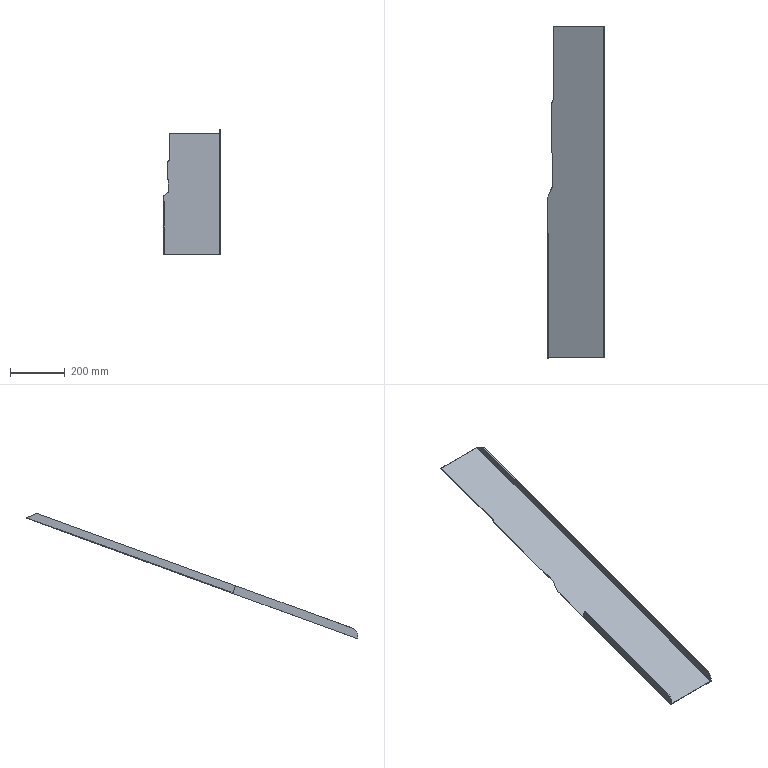Part | NX | features solid 2 | 1 solid | 19 faces | box 207.291 x 1212 x 458.334 mm | volume 602164 mm3 | plane 15 | spline 2 | cylinder 2 | commonest cylinder face diameters 60 x2